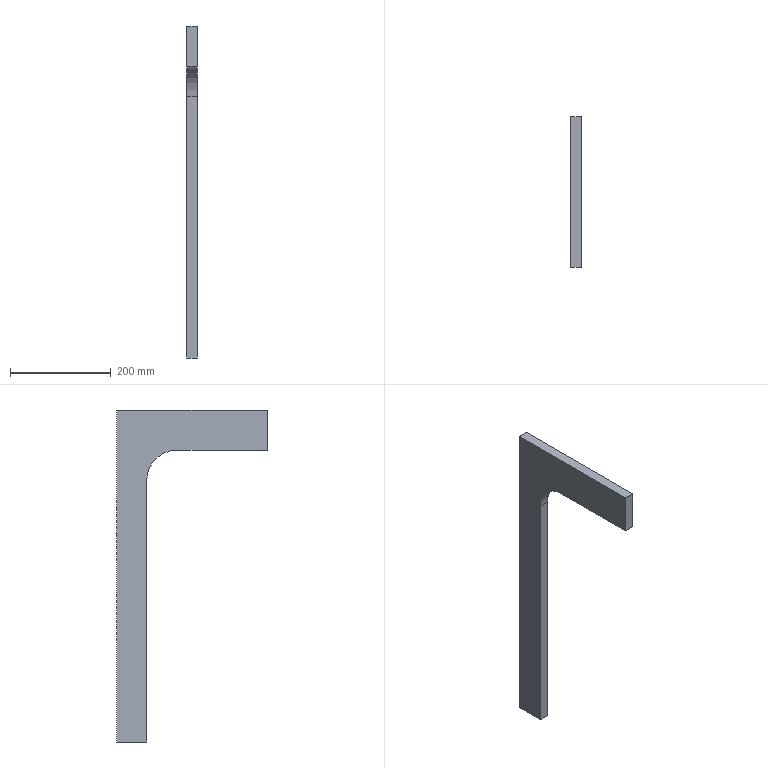Part | SolidWorks | features Extrusion 1, Fillet 1, ICE 1 | 1 solid | 9 faces | box 20 x 300 x 660 mm | volume 1191451 mm3 | plane 8 | cylinder 1 | commonest cylinder face diameters 120 x1
STEP:
#1=CARTESIAN_POINT('',(10.,-150.,330.));
#2=VERTEX_POINT('',#1);
#3=CARTESIAN_POINT('',(10.,-150.,250.));
#4=VERTEX_POINT('',#3);
#5=CARTESIAN_POINT('',(10.,-150.,330.));
#6=DIRECTION('',(0.,0.,-1.));
#7=VECTOR('',#6,1000.);
#8=LINE('',#5,#7);
#9=EDGE_CURVE('',#2,#4,#8,.T.);
#10=ORIENTED_EDGE('',*,*,#9,.T.);
#11=CARTESIAN_POINT('',(10.,30.,250.));
#12=VERTEX_POINT('',#11);
#13=CARTESIAN_POINT('',(10.,90.,250.));
#14=DIRECTION('',(0.,-1.,0.));
#15=VECTOR('',#14,1000.);
#16=LINE('',#13,#15);
#17=EDGE_CURVE('',#12,#4,#16,.T.);
#18=ORIENTED_EDGE('',*,*,#17,.F.);
#19=CARTESIAN_POINT('',(10.,90.,190.));
#20=VERTEX_POINT('',#19);
#21=CARTESIAN_POINT('',(10.,30.,190.));
#22=DIRECTION('',(-1.,0.,0.));
#23=DIRECTION('',(0.,0.,1.));
#24=AXIS2_PLACEMENT_3D('',#21,#22,#23);
#25=CIRCLE('',#24,60.);
#26=EDGE_CURVE('',#12,#20,#25,.T.);
#27=ORIENTED_EDGE('',*,*,#26,.T.);
#28=CARTESIAN_POINT('',(10.,90.,-330.));
#29=VERTEX_POINT('',#28);
#30=CARTESIAN_POINT('',(10.,90.,-330.));
#31=DIRECTION('',(0.,0.,1.));
#32=VECTOR('',#31,1000.);
#33=LINE('',#30,#32);
#34=EDGE_CURVE('',#29,#20,#33,.T.);
#35=ORIENTED_EDGE('',*,*,#34,.F.);
#36=CARTESIAN_POINT('',(10.,150.,-330.));
#37=VERTEX_POINT('',#36);
#38=CARTESIAN_POINT('',(10.,-150.,-330.));
#39=DIRECTION('',(0.,1.,0.));
#40=VECTOR('',#39,1000.);
#41=LINE('',#38,#40);
#42=EDGE_CURVE('',#29,#37,#41,.T.);
#43=ORIENTED_EDGE('',*,*,#42,.T.);
#44=CARTESIAN_POINT('',(10.,150.,330.));
#45=VERTEX_POINT('',#44);
#46=CARTESIAN_POINT('',(10.,150.,330.));
#47=DIRECTION('',(0.,0.,-1.));
#48=VECTOR('',#47,1000.);
#49=LINE('',#46,#48);
#50=EDGE_CURVE('',#45,#37,#49,.T.);
#51=ORIENTED_EDGE('',*,*,#50,.F.);
#52=CARTESIAN_POINT('',(10.,-150.,330.));
#53=DIRECTION('',(0.,1.,0.));
#54=VECTOR('',#53,1000.);
#55=LINE('',#52,#54);
#56=EDGE_CURVE('',#2,#45,#55,.T.);
#57=ORIENTED_EDGE('',*,*,#56,.F.);
#58=EDGE_LOOP('',(#10,#18,#27,#35,#43,#51,#57));
#59=FACE_OUTER_BOUND('',#58,.T.);
#60=CARTESIAN_POINT('',(10.,-150.,330.));
#61=DIRECTION('',(-1.,0.,0.));
#62=DIRECTION('',(0.,0.,1.));
#63=AXIS2_PLACEMENT_3D('',#60,#61,#62);
#64=PLANE('',#63);
#65=ADVANCED_FACE('',(#59),#64,.F.);
#66=CARTESIAN_POINT('',(-10.,150.,-330.));
#67=VERTEX_POINT('',#66);
#68=CARTESIAN_POINT('',(-10.,150.,-330.));
#69=DIRECTION('',(-1.,0.,0.));
#70=VECTOR('',#69,1000.);
#71=LINE('',#68,#70);
#72=EDGE_CURVE('',#37,#67,#71,.T.);
#73=ORIENTED_EDGE('',*,*,#72,.T.);
#74=CARTESIAN_POINT('',(-10.,150.,330.));
#75=VERTEX_POINT('',#74);
#76=CARTESIAN_POINT('',(-10.,150.,330.));
#77=DIRECTION('',(0.,0.,-1.));
#78=VECTOR('',#77,1000.);
#79=LINE('',#76,#78);
#80=EDGE_CURVE('',#75,#67,#79,.T.);
#81=ORIENTED_EDGE('',*,*,#80,.F.);
#82=CARTESIAN_POINT('',(-10.,150.,330.));
#83=DIRECTION('',(-1.,0.,0.));
#84=VECTOR('',#83,1000.);
#85=LINE('',#82,#84);
#86=EDGE_CURVE('',#45,#75,#85,.T.);
#87=ORIENTED_EDGE('',*,*,#86,.F.);
#88=ORIENTED_EDGE('',*,*,#50,.T.);
#89=EDGE_LOOP('',(#73,#81,#87,#88));
#90=FACE_OUTER_BOUND('',#89,.T.);
#91=CARTESIAN_POINT('',(-10.,150.,330.));
#92=DIRECTION('',(0.,-1.,0.));
#93=DIRECTION('',(0.,0.,-1.));
#94=AXIS2_PLACEMENT_3D('',#91,#92,#93);
#95=PLANE('',#94);
#96=ADVANCED_FACE('',(#90),#95,.F.);
#97=CARTESIAN_POINT('',(-10.,90.,-330.));
#98=VERTEX_POINT('',#97);
#99=CARTESIAN_POINT('',(-10.,90.,190.));
#100=VERTEX_POINT('',#99);
#101=CARTESIAN_POINT('',(-10.,90.,-330.));
#102=DIRECTION('',(0.,0.,1.));
#103=VECTOR('',#102,1000.);
#104=LINE('',#101,#103);
#105=EDGE_CURVE('',#98,#100,#104,.T.);
#106=ORIENTED_EDGE('',*,*,#105,.T.);
#107=CARTESIAN_POINT('',(-10.,30.,250.));
#108=VERTEX_POINT('',#107);
#109=CARTESIAN_POINT('',(-10.,30.,190.));
#110=DIRECTION('',(1.,0.,0.));
#111=DIRECTION('',(0.,0.,-1.));
#112=AXIS2_PLACEMENT_3D('',#109,#110,#111);
#113=CIRCLE('',#112,60.);
#114=EDGE_CURVE('',#100,#108,#113,.T.);
#115=ORIENTED_EDGE('',*,*,#114,.T.);
#116=CARTESIAN_POINT('',(-10.,-150.,250.));
#117=VERTEX_POINT('',#116);
#118=CARTESIAN_POINT('',(-10.,90.,250.));
#119=DIRECTION('',(0.,-1.,0.));
#120=VECTOR('',#119,1000.);
#121=LINE('',#118,#120);
#122=EDGE_CURVE('',#108,#117,#121,.T.);
#123=ORIENTED_EDGE('',*,*,#122,.T.);
#124=CARTESIAN_POINT('',(-10.,-150.,330.));
#125=VERTEX_POINT('',#124);
#126=CARTESIAN_POINT('',(-10.,-150.,330.));
#127=DIRECTION('',(0.,0.,-1.));
#128=VECTOR('',#127,1000.);
#129=LINE('',#126,#128);
#130=EDGE_CURVE('',#125,#117,#129,.T.);
#131=ORIENTED_EDGE('',*,*,#130,.F.);
#132=CARTESIAN_POINT('',(-10.,-150.,330.));
#133=DIRECTION('',(0.,-1.,0.));
#134=VECTOR('',#133,1000.);
#135=LINE('',#132,#134);
#136=EDGE_CURVE('',#75,#125,#135,.T.);
#137=ORIENTED_EDGE('',*,*,#136,.F.);
#138=ORIENTED_EDGE('',*,*,#80,.T.);
#139=CARTESIAN_POINT('',(-10.,-150.,-330.));
#140=DIRECTION('',(0.,-1.,0.));
#141=VECTOR('',#140,1000.);
#142=LINE('',#139,#141);
#143=EDGE_CURVE('',#67,#98,#142,.T.);
#144=ORIENTED_EDGE('',*,*,#143,.T.);
#145=EDGE_LOOP('',(#106,#115,#123,#131,#137,#138,#144));
#146=FACE_OUTER_BOUND('',#145,.T.);
#147=CARTESIAN_POINT('',(-10.,-150.,330.));
#148=DIRECTION('',(1.,0.,0.));
#149=DIRECTION('',(0.,0.,-1.));
#150=AXIS2_PLACEMENT_3D('',#147,#148,#149);
#151=PLANE('',#150);
#152=ADVANCED_FACE('',(#146),#151,.F.);
#153=ORIENTED_EDGE('',*,*,#130,.T.);
#154=CARTESIAN_POINT('',(-10.,-150.,250.));
#155=DIRECTION('',(1.,0.,0.));
#156=VECTOR('',#155,1000.);
#157=LINE('',#154,#156);
#158=EDGE_CURVE('',#117,#4,#157,.T.);
#159=ORIENTED_EDGE('',*,*,#158,.T.);
#160=ORIENTED_EDGE('',*,*,#9,.F.);
#161=CARTESIAN_POINT('',(-10.,-150.,330.));
#162=DIRECTION('',(1.,0.,0.));
#163=VECTOR('',#162,1000.);
#164=LINE('',#161,#163);
#165=EDGE_CURVE('',#125,#2,#164,.T.);
#166=ORIENTED_EDGE('',*,*,#165,.F.);
#167=EDGE_LOOP('',(#153,#159,#160,#166));
#168=FACE_OUTER_BOUND('',#167,.T.);
#169=CARTESIAN_POINT('',(-10.,-150.,330.));
#170=DIRECTION('',(0.,1.,0.));
#171=DIRECTION('',(0.,0.,1.));
#172=AXIS2_PLACEMENT_3D('',#169,#170,#171);
#173=PLANE('',#172);
#174=ADVANCED_FACE('',(#168),#173,.F.);
#175=ORIENTED_EDGE('',*,*,#56,.T.);
#176=ORIENTED_EDGE('',*,*,#86,.T.);
#177=ORIENTED_EDGE('',*,*,#136,.T.);
#178=ORIENTED_EDGE('',*,*,#165,.T.);
#179=EDGE_LOOP('',(#175,#176,#177,#178));
#180=FACE_OUTER_BOUND('',#179,.T.);
#181=CARTESIAN_POINT('',(0.,0.,330.));
#182=DIRECTION('',(0.,0.,-1.));
#183=DIRECTION('',(-1.,0.,0.));
#184=AXIS2_PLACEMENT_3D('',#181,#182,#183);
#185=PLANE('',#184);
#186=ADVANCED_FACE('',(#180),#185,.F.);
#187=CARTESIAN_POINT('',(-10.,90.,-330.));
#188=DIRECTION('',(1.,0.,0.));
#189=VECTOR('',#188,1000.);
#190=LINE('',#187,#189);
#191=EDGE_CURVE('',#98,#29,#190,.T.);
#192=ORIENTED_EDGE('',*,*,#191,.F.);
#193=ORIENTED_EDGE('',*,*,#143,.F.);
#194=ORIENTED_EDGE('',*,*,#72,.F.);
#195=ORIENTED_EDGE('',*,*,#42,.F.);
#196=EDGE_LOOP('',(#192,#193,#194,#195));
#197=FACE_OUTER_BOUND('',#196,.T.);
#198=CARTESIAN_POINT('',(0.,0.,-330.));
#199=DIRECTION('',(0.,0.,-1.));
#200=DIRECTION('',(-1.,0.,0.));
#201=AXIS2_PLACEMENT_3D('',#198,#199,#200);
#202=PLANE('',#201);
#203=ADVANCED_FACE('',(#197),#202,.T.);
#204=ORIENTED_EDGE('',*,*,#122,.F.);
#205=CARTESIAN_POINT('',(10.,30.,250.));
#206=DIRECTION('',(1.,0.,0.));
#207=VECTOR('',#206,1000.);
#208=LINE('',#205,#207);
#209=EDGE_CURVE('',#108,#12,#208,.T.);
#210=ORIENTED_EDGE('',*,*,#209,.T.);
#211=ORIENTED_EDGE('',*,*,#17,.T.);
#212=ORIENTED_EDGE('',*,*,#158,.F.);
#213=EDGE_LOOP('',(#204,#210,#211,#212));
#214=FACE_OUTER_BOUND('',#213,.T.);
#215=CARTESIAN_POINT('',(-10.,90.,250.));
#216=DIRECTION('',(0.,0.,1.));
#217=DIRECTION('',(0.,-1.,0.));
#218=AXIS2_PLACEMENT_3D('',#215,#216,#217);
#219=PLANE('',#218);
#220=ADVANCED_FACE('',(#214),#219,.F.);
#221=ORIENTED_EDGE('',*,*,#34,.T.);
#222=CARTESIAN_POINT('',(-10.,90.,190.));
#223=DIRECTION('',(-1.,0.,0.));
#224=VECTOR('',#223,1000.);
#225=LINE('',#222,#224);
#226=EDGE_CURVE('',#20,#100,#225,.T.);
#227=ORIENTED_EDGE('',*,*,#226,.T.);
#228=ORIENTED_EDGE('',*,*,#105,.F.);
#229=ORIENTED_EDGE('',*,*,#191,.T.);
#230=EDGE_LOOP('',(#221,#227,#228,#229));
#231=FACE_OUTER_BOUND('',#230,.T.);
#232=CARTESIAN_POINT('',(-10.,90.,-330.));
#233=DIRECTION('',(0.,1.,0.));
#234=DIRECTION('',(0.,0.,1.));
#235=AXIS2_PLACEMENT_3D('',#232,#233,#234);
#236=PLANE('',#235);
#237=ADVANCED_FACE('',(#231),#236,.F.);
#238=ORIENTED_EDGE('',*,*,#114,.F.);
#239=ORIENTED_EDGE('',*,*,#226,.F.);
#240=ORIENTED_EDGE('',*,*,#26,.F.);
#241=ORIENTED_EDGE('',*,*,#209,.F.);
#242=EDGE_LOOP('',(#238,#239,#240,#241));
#243=FACE_OUTER_BOUND('',#242,.T.);
#244=CARTESIAN_POINT('',(-10.,30.,190.));
#245=DIRECTION('',(-1.,0.,0.));
#246=DIRECTION('',(0.,0.,1.));
#247=AXIS2_PLACEMENT_3D('',#244,#245,#246);
#248=CYLINDRICAL_SURFACE('',#247,60.);
#249=ADVANCED_FACE('',(#243),#248,.F.);
#250=CLOSED_SHELL('',(#65,#96,#152,#174,#186,#203,#220,#237,#249));
#251=MANIFOLD_SOLID_BREP('',#250);
#252=CARTESIAN_POINT('',(0.,0.,0.));
#253=DIRECTION('',(0.,0.,1.));
#254=DIRECTION('',(1.,0.,0.));
#255=AXIS2_PLACEMENT_3D('',#252,#253,#254);
#256=(LENGTH_UNIT()NAMED_UNIT(*)SI_UNIT(.MILLI.,.METRE.));
#257=UNCERTAINTY_MEASURE_WITH_UNIT(LENGTH_MEASURE(0.00001),#256,'','');
#258=(NAMED_UNIT(*)PLANE_ANGLE_UNIT()SI_UNIT($,.RADIAN.));
#259=(NAMED_UNIT(*)SI_UNIT($,.STERADIAN.)SOLID_ANGLE_UNIT());
#260=(GEOMETRIC_REPRESENTATION_CONTEXT(3)GLOBAL_UNCERTAINTY_ASSIGNED_CONTEXT((#257))GLOBAL_UNIT_ASSIGNED_CONTEXT((#256,#258,#259))REPRESENTATION_CONTEXT('',''));
#261=ADVANCED_BREP_SHAPE_REPRESENTATION('',(#251,#255),#260);